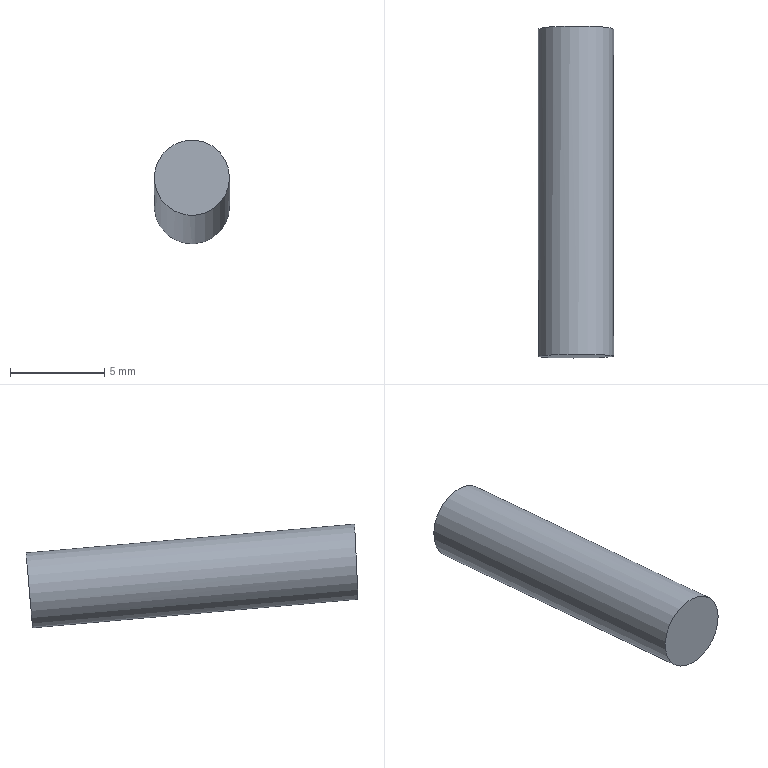Part | NX | features solid 2 | 1 solid | 3 faces | box 4 x 17.645 x 5.513 mm | volume 219.232 mm3 | plane 2 | cylinder 1 | commonest cylinder face diameters 4 x1
STEP:
#1=CARTESIAN_POINT('',(-105.455,-29.15,-40.641));
#2=VERTEX_POINT('',#1);
#3=CARTESIAN_POINT('',(-105.455,-28.975,-38.649));
#4=DIRECTION('',(0.,-0.9962,0.08716));
#5=DIRECTION('',(0.,-0.08716,-0.9962));
#6=AXIS2_PLACEMENT_3D('',#3,#4,#5);
#7=CIRCLE('',#6,2.);
#8=EDGE_CURVE('',#2,#2,#7,.T.);
#9=ORIENTED_EDGE('',*,*,#8,.F.);
#10=EDGE_LOOP('',(#9));
#11=FACE_BOUND('',#10,.T.);
#12=CARTESIAN_POINT('',(-105.455,-28.975,-38.649));
#13=DIRECTION('',(0.,0.9962,-0.08716));
#14=DIRECTION('',(0.,0.08716,0.9962));
#15=AXIS2_PLACEMENT_3D('',#12,#13,#14);
#16=PLANE('',#15);
#17=ADVANCED_FACE('',(#11),#16,.T.);
#18=CARTESIAN_POINT('',(-105.269,-46.445,-39.119));
#19=VERTEX_POINT('',#18);
#20=CARTESIAN_POINT('',(-105.455,-46.355,-37.128));
#21=DIRECTION('',(0.00391,-0.999,0.04549));
#22=DIRECTION('',(0.09317,-0.04493,-0.9946));
#23=AXIS2_PLACEMENT_3D('',#20,#21,#22);
#24=ELLIPSE('',#23,2.002,2.);
#25=EDGE_CURVE('',#19,#19,#24,.F.);
#26=ORIENTED_EDGE('',*,*,#25,.F.);
#27=EDGE_LOOP('',(#26));
#28=FACE_BOUND('',#27,.T.);
#29=CARTESIAN_POINT('',(-78.701,-48.763,-92.296));
#30=DIRECTION('',(0.00391,-0.999,0.04549));
#31=DIRECTION('',(-0.05224,0.04523,0.9976));
#32=AXIS2_PLACEMENT_3D('',#29,#30,#31);
#33=PLANE('',#32);
#34=ADVANCED_FACE('',(#28),#33,.T.);
#35=ORIENTED_EDGE('',*,*,#8,.T.);
#36=EDGE_LOOP('',(#35));
#37=FACE_BOUND('',#36,.T.);
#38=ORIENTED_EDGE('',*,*,#25,.T.);
#39=EDGE_LOOP('',(#38));
#40=FACE_BOUND('',#39,.T.);
#41=CARTESIAN_POINT('',(-105.455,-48.899,-36.906));
#42=DIRECTION('',(0.,0.9962,-0.08716));
#43=DIRECTION('',(0.,0.08716,0.9962));
#44=AXIS2_PLACEMENT_3D('',#41,#42,#43);
#45=CYLINDRICAL_SURFACE('',#44,2.);
#46=ADVANCED_FACE('',(#37,#40),#45,.T.);
#47=CLOSED_SHELL('',(#17,#34,#46));
#48=MANIFOLD_SOLID_BREP('',#47);
#49=(LENGTH_UNIT()NAMED_UNIT(*)SI_UNIT(.MILLI.,.METRE.));
#50=UNCERTAINTY_MEASURE_WITH_UNIT(LENGTH_MEASURE(0.00001),#49,'','');
#51=(NAMED_UNIT(*)PLANE_ANGLE_UNIT()SI_UNIT($,.RADIAN.));
#52=(NAMED_UNIT(*)SI_UNIT($,.STERADIAN.)SOLID_ANGLE_UNIT());
#53=(GEOMETRIC_REPRESENTATION_CONTEXT(3)GLOBAL_UNCERTAINTY_ASSIGNED_CONTEXT((#50))GLOBAL_UNIT_ASSIGNED_CONTEXT((#49,#51,#52))REPRESENTATION_CONTEXT('',''));
#54=ADVANCED_BREP_SHAPE_REPRESENTATION('',(#48),#53);